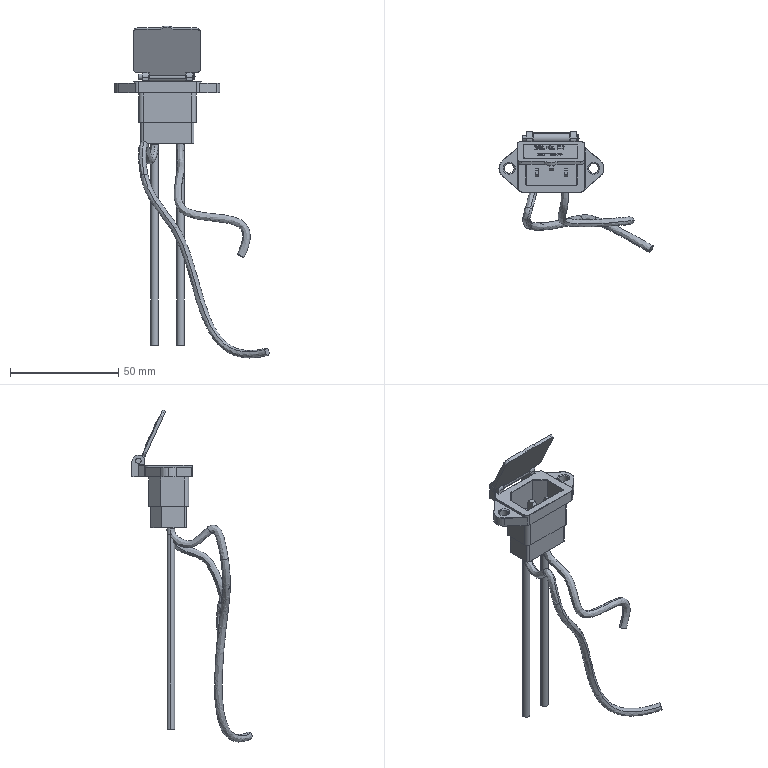Part | SolidWorks | 7 solids | 443 faces | box 71.171 x 55.586 x 153.356 mm | volume 14195 mm3 | plane 282 | spline 73 | cylinder 71 | torus 11 | cone 4 | sphere 2 | commonest cylinder face diameters 0.2 x20 4 x10 2.5 x8 3.5 x8 2 x6 4.5 x4